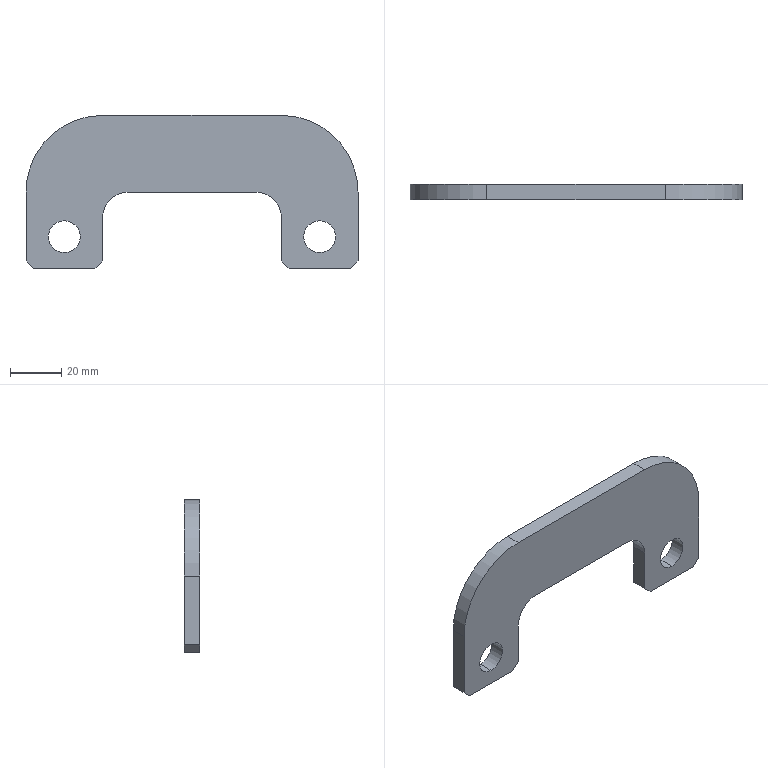Part | SolidWorks | features FlatPattern 1, SMBaseFlange 1, SheetMetal 1 | 1 solid | 22 faces | box 130 x 6 x 60 mm | volume 30559 mm3 | plane 14 | cylinder 8 | commonest cylinder face diameters 12.5 x4 20 x2 60 x2
STEP:
#1=CARTESIAN_POINT('',(15.,-6.,6.25));
#2=VERTEX_POINT('',#1);
#3=CARTESIAN_POINT('',(15.,-6.,18.75));
#4=VERTEX_POINT('',#3);
#5=CARTESIAN_POINT('',(15.,-6.,12.5));
#6=DIRECTION('',(0.,1.,0.));
#7=DIRECTION('',(0.,0.,1.));
#8=AXIS2_PLACEMENT_3D('',#5,#6,#7);
#9=CIRCLE('',#8,6.25);
#10=EDGE_CURVE('',#2,#4,#9,.T.);
#11=ORIENTED_EDGE('',*,*,#10,.F.);
#12=CARTESIAN_POINT('',(15.,0.,6.25));
#13=VERTEX_POINT('',#12);
#14=CARTESIAN_POINT('',(15.,-6.,6.25));
#15=DIRECTION('',(0.,1.,0.));
#16=VECTOR('',#15,1000.);
#17=LINE('',#14,#16);
#18=EDGE_CURVE('',#2,#13,#17,.T.);
#19=ORIENTED_EDGE('',*,*,#18,.T.);
#20=CARTESIAN_POINT('',(15.,0.,18.75));
#21=VERTEX_POINT('',#20);
#22=CARTESIAN_POINT('',(15.,0.,12.5));
#23=DIRECTION('',(0.,1.,0.));
#24=DIRECTION('',(0.,0.,1.));
#25=AXIS2_PLACEMENT_3D('',#22,#23,#24);
#26=CIRCLE('',#25,6.25);
#27=EDGE_CURVE('',#13,#21,#26,.T.);
#28=ORIENTED_EDGE('',*,*,#27,.T.);
#29=CARTESIAN_POINT('',(15.,-6.,18.75));
#30=DIRECTION('',(0.,1.,0.));
#31=VECTOR('',#30,1000.);
#32=LINE('',#29,#31);
#33=EDGE_CURVE('',#4,#21,#32,.T.);
#34=ORIENTED_EDGE('',*,*,#33,.F.);
#35=EDGE_LOOP('',(#11,#19,#28,#34));
#36=FACE_OUTER_BOUND('',#35,.T.);
#37=CARTESIAN_POINT('',(15.,-6.,12.5));
#38=DIRECTION('',(0.,1.,0.));
#39=DIRECTION('',(0.,0.,1.));
#40=AXIS2_PLACEMENT_3D('',#37,#38,#39);
#41=CYLINDRICAL_SURFACE('',#40,6.25);
#42=ADVANCED_FACE('',(#36),#41,.F.);
#43=CARTESIAN_POINT('',(115.,-6.,6.25));
#44=VERTEX_POINT('',#43);
#45=CARTESIAN_POINT('',(115.,-6.,18.75));
#46=VERTEX_POINT('',#45);
#47=CARTESIAN_POINT('',(115.,-6.,12.5));
#48=DIRECTION('',(0.,1.,0.));
#49=DIRECTION('',(0.,0.,1.));
#50=AXIS2_PLACEMENT_3D('',#47,#48,#49);
#51=CIRCLE('',#50,6.25);
#52=EDGE_CURVE('',#44,#46,#51,.T.);
#53=ORIENTED_EDGE('',*,*,#52,.F.);
#54=CARTESIAN_POINT('',(115.,0.,6.25));
#55=VERTEX_POINT('',#54);
#56=CARTESIAN_POINT('',(115.,-6.,6.25));
#57=DIRECTION('',(0.,1.,0.));
#58=VECTOR('',#57,1000.);
#59=LINE('',#56,#58);
#60=EDGE_CURVE('',#44,#55,#59,.T.);
#61=ORIENTED_EDGE('',*,*,#60,.T.);
#62=CARTESIAN_POINT('',(115.,0.,18.75));
#63=VERTEX_POINT('',#62);
#64=CARTESIAN_POINT('',(115.,0.,12.5));
#65=DIRECTION('',(0.,1.,0.));
#66=DIRECTION('',(0.,0.,1.));
#67=AXIS2_PLACEMENT_3D('',#64,#65,#66);
#68=CIRCLE('',#67,6.25);
#69=EDGE_CURVE('',#55,#63,#68,.T.);
#70=ORIENTED_EDGE('',*,*,#69,.T.);
#71=CARTESIAN_POINT('',(115.,-6.,18.75));
#72=DIRECTION('',(0.,1.,0.));
#73=VECTOR('',#72,1000.);
#74=LINE('',#71,#73);
#75=EDGE_CURVE('',#46,#63,#74,.T.);
#76=ORIENTED_EDGE('',*,*,#75,.F.);
#77=EDGE_LOOP('',(#53,#61,#70,#76));
#78=FACE_OUTER_BOUND('',#77,.T.);
#79=CARTESIAN_POINT('',(115.,-6.,12.5));
#80=DIRECTION('',(0.,1.,0.));
#81=DIRECTION('',(0.,0.,1.));
#82=AXIS2_PLACEMENT_3D('',#79,#80,#81);
#83=CYLINDRICAL_SURFACE('',#82,6.25);
#84=ADVANCED_FACE('',(#78),#83,.F.);
#85=CARTESIAN_POINT('',(100.,0.,20.));
#86=VERTEX_POINT('',#85);
#87=CARTESIAN_POINT('',(90.,0.,30.));
#88=VERTEX_POINT('',#87);
#89=CARTESIAN_POINT('',(90.,0.,20.));
#90=DIRECTION('',(0.,-1.,0.));
#91=DIRECTION('',(0.,0.,-1.));
#92=AXIS2_PLACEMENT_3D('',#89,#90,#91);
#93=CIRCLE('',#92,10.);
#94=EDGE_CURVE('',#86,#88,#93,.T.);
#95=ORIENTED_EDGE('',*,*,#94,.F.);
#96=CARTESIAN_POINT('',(100.,-6.,20.));
#97=VERTEX_POINT('',#96);
#98=CARTESIAN_POINT('',(100.,-6.,20.));
#99=DIRECTION('',(0.,1.,0.));
#100=VECTOR('',#99,1000.);
#101=LINE('',#98,#100);
#102=EDGE_CURVE('',#97,#86,#101,.T.);
#103=ORIENTED_EDGE('',*,*,#102,.F.);
#104=CARTESIAN_POINT('',(90.,-6.,30.));
#105=VERTEX_POINT('',#104);
#106=CARTESIAN_POINT('',(90.,-6.,20.));
#107=DIRECTION('',(0.,-1.,0.));
#108=DIRECTION('',(0.,0.,-1.));
#109=AXIS2_PLACEMENT_3D('',#106,#107,#108);
#110=CIRCLE('',#109,10.);
#111=EDGE_CURVE('',#97,#105,#110,.T.);
#112=ORIENTED_EDGE('',*,*,#111,.T.);
#113=CARTESIAN_POINT('',(90.,-6.,30.));
#114=DIRECTION('',(0.,1.,0.));
#115=VECTOR('',#114,1000.);
#116=LINE('',#113,#115);
#117=EDGE_CURVE('',#105,#88,#116,.T.);
#118=ORIENTED_EDGE('',*,*,#117,.T.);
#119=EDGE_LOOP('',(#95,#103,#112,#118));
#120=FACE_OUTER_BOUND('',#119,.T.);
#121=CARTESIAN_POINT('',(90.,-6.,20.));
#122=DIRECTION('',(0.,1.,0.));
#123=DIRECTION('',(0.,0.,1.));
#124=AXIS2_PLACEMENT_3D('',#121,#122,#123);
#125=CYLINDRICAL_SURFACE('',#124,10.);
#126=ADVANCED_FACE('',(#120),#125,.F.);
#127=CARTESIAN_POINT('',(100.,0.,3.));
#128=VERTEX_POINT('',#127);
#129=CARTESIAN_POINT('',(100.,0.,3.));
#130=DIRECTION('',(0.,0.,1.));
#131=VECTOR('',#130,1000.);
#132=LINE('',#129,#131);
#133=EDGE_CURVE('',#128,#86,#132,.T.);
#134=ORIENTED_EDGE('',*,*,#133,.F.);
#135=CARTESIAN_POINT('',(100.,-6.,3.));
#136=VERTEX_POINT('',#135);
#137=CARTESIAN_POINT('',(100.,-6.,3.));
#138=DIRECTION('',(0.,1.,0.));
#139=VECTOR('',#138,1000.);
#140=LINE('',#137,#139);
#141=EDGE_CURVE('',#136,#128,#140,.T.);
#142=ORIENTED_EDGE('',*,*,#141,.F.);
#143=CARTESIAN_POINT('',(100.,-6.,3.));
#144=DIRECTION('',(0.,0.,1.));
#145=VECTOR('',#144,1000.);
#146=LINE('',#143,#145);
#147=EDGE_CURVE('',#136,#97,#146,.T.);
#148=ORIENTED_EDGE('',*,*,#147,.T.);
#149=ORIENTED_EDGE('',*,*,#102,.T.);
#150=EDGE_LOOP('',(#134,#142,#148,#149));
#151=FACE_OUTER_BOUND('',#150,.T.);
#152=CARTESIAN_POINT('',(100.,-6.,3.));
#153=DIRECTION('',(-1.,0.,0.));
#154=DIRECTION('',(0.,0.,1.));
#155=AXIS2_PLACEMENT_3D('',#152,#153,#154);
#156=PLANE('',#155);
#157=ADVANCED_FACE('',(#151),#156,.T.);
#158=CARTESIAN_POINT('',(103.,0.,0.));
#159=VERTEX_POINT('',#158);
#160=CARTESIAN_POINT('',(103.,0.,0.));
#161=DIRECTION('',(-0.7071,0.,0.7071));
#162=VECTOR('',#161,1000.);
#163=LINE('',#160,#162);
#164=EDGE_CURVE('',#159,#128,#163,.T.);
#165=ORIENTED_EDGE('',*,*,#164,.F.);
#166=CARTESIAN_POINT('',(103.,-6.,0.));
#167=VERTEX_POINT('',#166);
#168=CARTESIAN_POINT('',(103.,-6.,0.));
#169=DIRECTION('',(0.,1.,0.));
#170=VECTOR('',#169,1000.);
#171=LINE('',#168,#170);
#172=EDGE_CURVE('',#167,#159,#171,.T.);
#173=ORIENTED_EDGE('',*,*,#172,.F.);
#174=CARTESIAN_POINT('',(103.,-6.,0.));
#175=DIRECTION('',(-0.7071,0.,0.7071));
#176=VECTOR('',#175,1000.);
#177=LINE('',#174,#176);
#178=EDGE_CURVE('',#167,#136,#177,.T.);
#179=ORIENTED_EDGE('',*,*,#178,.T.);
#180=ORIENTED_EDGE('',*,*,#141,.T.);
#181=EDGE_LOOP('',(#165,#173,#179,#180));
#182=FACE_OUTER_BOUND('',#181,.T.);
#183=CARTESIAN_POINT('',(103.,-6.,0.));
#184=DIRECTION('',(-0.7071,0.,-0.7071));
#185=DIRECTION('',(-0.7071,0.,0.7071));
#186=AXIS2_PLACEMENT_3D('',#183,#184,#185);
#187=PLANE('',#186);
#188=ADVANCED_FACE('',(#182),#187,.T.);
#189=CARTESIAN_POINT('',(127.,0.,0.));
#190=VERTEX_POINT('',#189);
#191=CARTESIAN_POINT('',(127.,0.,0.));
#192=DIRECTION('',(-1.,0.,0.));
#193=VECTOR('',#192,1000.);
#194=LINE('',#191,#193);
#195=EDGE_CURVE('',#190,#159,#194,.T.);
#196=ORIENTED_EDGE('',*,*,#195,.F.);
#197=CARTESIAN_POINT('',(127.,-6.,0.));
#198=VERTEX_POINT('',#197);
#199=CARTESIAN_POINT('',(127.,-6.,0.));
#200=DIRECTION('',(0.,1.,0.));
#201=VECTOR('',#200,1000.);
#202=LINE('',#199,#201);
#203=EDGE_CURVE('',#198,#190,#202,.T.);
#204=ORIENTED_EDGE('',*,*,#203,.F.);
#205=CARTESIAN_POINT('',(127.,-6.,0.));
#206=DIRECTION('',(-1.,0.,0.));
#207=VECTOR('',#206,1000.);
#208=LINE('',#205,#207);
#209=EDGE_CURVE('',#198,#167,#208,.T.);
#210=ORIENTED_EDGE('',*,*,#209,.T.);
#211=ORIENTED_EDGE('',*,*,#172,.T.);
#212=EDGE_LOOP('',(#196,#204,#210,#211));
#213=FACE_OUTER_BOUND('',#212,.T.);
#214=CARTESIAN_POINT('',(127.,-6.,0.));
#215=DIRECTION('',(0.,0.,-1.));
#216=DIRECTION('',(-1.,0.,0.));
#217=AXIS2_PLACEMENT_3D('',#214,#215,#216);
#218=PLANE('',#217);
#219=ADVANCED_FACE('',(#213),#218,.T.);
#220=CARTESIAN_POINT('',(130.,0.,3.));
#221=VERTEX_POINT('',#220);
#222=CARTESIAN_POINT('',(130.,0.,3.));
#223=DIRECTION('',(-0.7071,0.,-0.7071));
#224=VECTOR('',#223,1000.);
#225=LINE('',#222,#224);
#226=EDGE_CURVE('',#221,#190,#225,.T.);
#227=ORIENTED_EDGE('',*,*,#226,.F.);
#228=CARTESIAN_POINT('',(130.,-6.,3.));
#229=VERTEX_POINT('',#228);
#230=CARTESIAN_POINT('',(130.,-6.,3.));
#231=DIRECTION('',(0.,1.,0.));
#232=VECTOR('',#231,1000.);
#233=LINE('',#230,#232);
#234=EDGE_CURVE('',#229,#221,#233,.T.);
#235=ORIENTED_EDGE('',*,*,#234,.F.);
#236=CARTESIAN_POINT('',(130.,-6.,3.));
#237=DIRECTION('',(-0.7071,0.,-0.7071));
#238=VECTOR('',#237,1000.);
#239=LINE('',#236,#238);
#240=EDGE_CURVE('',#229,#198,#239,.T.);
#241=ORIENTED_EDGE('',*,*,#240,.T.);
#242=ORIENTED_EDGE('',*,*,#203,.T.);
#243=EDGE_LOOP('',(#227,#235,#241,#242));
#244=FACE_OUTER_BOUND('',#243,.T.);
#245=CARTESIAN_POINT('',(130.,-6.,3.));
#246=DIRECTION('',(0.7071,0.,-0.7071));
#247=DIRECTION('',(-0.7071,0.,-0.7071));
#248=AXIS2_PLACEMENT_3D('',#245,#246,#247);
#249=PLANE('',#248);
#250=ADVANCED_FACE('',(#244),#249,.T.);
#251=CARTESIAN_POINT('',(130.,0.,30.));
#252=VERTEX_POINT('',#251);
#253=CARTESIAN_POINT('',(130.,0.,30.));
#254=DIRECTION('',(0.,0.,-1.));
#255=VECTOR('',#254,1000.);
#256=LINE('',#253,#255);
#257=EDGE_CURVE('',#252,#221,#256,.T.);
#258=ORIENTED_EDGE('',*,*,#257,.F.);
#259=CARTESIAN_POINT('',(130.,-6.,30.));
#260=VERTEX_POINT('',#259);
#261=CARTESIAN_POINT('',(130.,-6.,30.));
#262=DIRECTION('',(0.,1.,0.));
#263=VECTOR('',#262,1000.);
#264=LINE('',#261,#263);
#265=EDGE_CURVE('',#260,#252,#264,.T.);
#266=ORIENTED_EDGE('',*,*,#265,.F.);
#267=CARTESIAN_POINT('',(130.,-6.,30.));
#268=DIRECTION('',(0.,0.,-1.));
#269=VECTOR('',#268,1000.);
#270=LINE('',#267,#269);
#271=EDGE_CURVE('',#260,#229,#270,.T.);
#272=ORIENTED_EDGE('',*,*,#271,.T.);
#273=ORIENTED_EDGE('',*,*,#234,.T.);
#274=EDGE_LOOP('',(#258,#266,#272,#273));
#275=FACE_OUTER_BOUND('',#274,.T.);
#276=CARTESIAN_POINT('',(130.,-6.,30.));
#277=DIRECTION('',(1.,0.,0.));
#278=DIRECTION('',(0.,0.,-1.));
#279=AXIS2_PLACEMENT_3D('',#276,#277,#278);
#280=PLANE('',#279);
#281=ADVANCED_FACE('',(#275),#280,.T.);
#282=CARTESIAN_POINT('',(100.,0.,60.));
#283=VERTEX_POINT('',#282);
#284=CARTESIAN_POINT('',(100.,0.,30.));
#285=DIRECTION('',(0.,1.,0.));
#286=DIRECTION('',(0.,0.,1.));
#287=AXIS2_PLACEMENT_3D('',#284,#285,#286);
#288=CIRCLE('',#287,30.);
#289=EDGE_CURVE('',#283,#252,#288,.T.);
#290=ORIENTED_EDGE('',*,*,#289,.F.);
#291=CARTESIAN_POINT('',(100.,-6.,60.));
#292=VERTEX_POINT('',#291);
#293=CARTESIAN_POINT('',(100.,-6.,60.));
#294=DIRECTION('',(0.,1.,0.));
#295=VECTOR('',#294,1000.);
#296=LINE('',#293,#295);
#297=EDGE_CURVE('',#292,#283,#296,.T.);
#298=ORIENTED_EDGE('',*,*,#297,.F.);
#299=CARTESIAN_POINT('',(100.,-6.,30.));
#300=DIRECTION('',(0.,1.,0.));
#301=DIRECTION('',(0.,0.,1.));
#302=AXIS2_PLACEMENT_3D('',#299,#300,#301);
#303=CIRCLE('',#302,30.);
#304=EDGE_CURVE('',#292,#260,#303,.T.);
#305=ORIENTED_EDGE('',*,*,#304,.T.);
#306=ORIENTED_EDGE('',*,*,#265,.T.);
#307=EDGE_LOOP('',(#290,#298,#305,#306));
#308=FACE_OUTER_BOUND('',#307,.T.);
#309=CARTESIAN_POINT('',(100.,-6.,30.));
#310=DIRECTION('',(0.,1.,0.));
#311=DIRECTION('',(0.,0.,1.));
#312=AXIS2_PLACEMENT_3D('',#309,#310,#311);
#313=CYLINDRICAL_SURFACE('',#312,30.);
#314=ADVANCED_FACE('',(#308),#313,.T.);
#315=CARTESIAN_POINT('',(30.,0.,60.));
#316=VERTEX_POINT('',#315);
#317=CARTESIAN_POINT('',(30.,0.,60.));
#318=DIRECTION('',(1.,0.,0.));
#319=VECTOR('',#318,1000.);
#320=LINE('',#317,#319);
#321=EDGE_CURVE('',#316,#283,#320,.T.);
#322=ORIENTED_EDGE('',*,*,#321,.F.);
#323=CARTESIAN_POINT('',(30.,-6.,60.));
#324=VERTEX_POINT('',#323);
#325=CARTESIAN_POINT('',(30.,-6.,60.));
#326=DIRECTION('',(0.,1.,0.));
#327=VECTOR('',#326,1000.);
#328=LINE('',#325,#327);
#329=EDGE_CURVE('',#324,#316,#328,.T.);
#330=ORIENTED_EDGE('',*,*,#329,.F.);
#331=CARTESIAN_POINT('',(30.,-6.,60.));
#332=DIRECTION('',(1.,0.,0.));
#333=VECTOR('',#332,1000.);
#334=LINE('',#331,#333);
#335=EDGE_CURVE('',#324,#292,#334,.T.);
#336=ORIENTED_EDGE('',*,*,#335,.T.);
#337=ORIENTED_EDGE('',*,*,#297,.T.);
#338=EDGE_LOOP('',(#322,#330,#336,#337));
#339=FACE_OUTER_BOUND('',#338,.T.);
#340=CARTESIAN_POINT('',(30.,-6.,60.));
#341=DIRECTION('',(0.,0.,1.));
#342=DIRECTION('',(1.,0.,0.));
#343=AXIS2_PLACEMENT_3D('',#340,#341,#342);
#344=PLANE('',#343);
#345=ADVANCED_FACE('',(#339),#344,.T.);
#346=CARTESIAN_POINT('',(0.,0.,30.));
#347=VERTEX_POINT('',#346);
#348=CARTESIAN_POINT('',(30.,0.,30.));
#349=DIRECTION('',(0.,1.,0.));
#350=DIRECTION('',(0.,0.,1.));
#351=AXIS2_PLACEMENT_3D('',#348,#349,#350);
#352=CIRCLE('',#351,30.);
#353=EDGE_CURVE('',#347,#316,#352,.T.);
#354=ORIENTED_EDGE('',*,*,#353,.F.);
#355=CARTESIAN_POINT('',(0.,-6.,30.));
#356=VERTEX_POINT('',#355);
#357=CARTESIAN_POINT('',(0.,-6.,30.));
#358=DIRECTION('',(0.,1.,0.));
#359=VECTOR('',#358,1000.);
#360=LINE('',#357,#359);
#361=EDGE_CURVE('',#356,#347,#360,.T.);
#362=ORIENTED_EDGE('',*,*,#361,.F.);
#363=CARTESIAN_POINT('',(30.,-6.,30.));
#364=DIRECTION('',(0.,1.,0.));
#365=DIRECTION('',(0.,0.,1.));
#366=AXIS2_PLACEMENT_3D('',#363,#364,#365);
#367=CIRCLE('',#366,30.);
#368=EDGE_CURVE('',#356,#324,#367,.T.);
#369=ORIENTED_EDGE('',*,*,#368,.T.);
#370=ORIENTED_EDGE('',*,*,#329,.T.);
#371=EDGE_LOOP('',(#354,#362,#369,#370));
#372=FACE_OUTER_BOUND('',#371,.T.);
#373=CARTESIAN_POINT('',(30.,-6.,30.));
#374=DIRECTION('',(0.,1.,0.));
#375=DIRECTION('',(0.,0.,1.));
#376=AXIS2_PLACEMENT_3D('',#373,#374,#375);
#377=CYLINDRICAL_SURFACE('',#376,30.);
#378=ADVANCED_FACE('',(#372),#377,.T.);
#379=CARTESIAN_POINT('',(0.,0.,3.));
#380=VERTEX_POINT('',#379);
#381=CARTESIAN_POINT('',(0.,0.,3.));
#382=DIRECTION('',(0.,0.,1.));
#383=VECTOR('',#382,1000.);
#384=LINE('',#381,#383);
#385=EDGE_CURVE('',#380,#347,#384,.T.);
#386=ORIENTED_EDGE('',*,*,#385,.F.);
#387=CARTESIAN_POINT('',(0.,-6.,3.));
#388=VERTEX_POINT('',#387);
#389=CARTESIAN_POINT('',(0.,-6.,3.));
#390=DIRECTION('',(0.,1.,0.));
#391=VECTOR('',#390,1000.);
#392=LINE('',#389,#391);
#393=EDGE_CURVE('',#388,#380,#392,.T.);
#394=ORIENTED_EDGE('',*,*,#393,.F.);
#395=CARTESIAN_POINT('',(0.,-6.,3.));
#396=DIRECTION('',(0.,0.,1.));
#397=VECTOR('',#396,1000.);
#398=LINE('',#395,#397);
#399=EDGE_CURVE('',#388,#356,#398,.T.);
#400=ORIENTED_EDGE('',*,*,#399,.T.);
#401=ORIENTED_EDGE('',*,*,#361,.T.);
#402=EDGE_LOOP('',(#386,#394,#400,#401));
#403=FACE_OUTER_BOUND('',#402,.T.);
#404=CARTESIAN_POINT('',(0.,-6.,3.));
#405=DIRECTION('',(-1.,0.,0.));
#406=DIRECTION('',(0.,0.,1.));
#407=AXIS2_PLACEMENT_3D('',#404,#405,#406);
#408=PLANE('',#407);
#409=ADVANCED_FACE('',(#403),#408,.T.);
#410=CARTESIAN_POINT('',(3.,0.,0.));
#411=VERTEX_POINT('',#410);
#412=CARTESIAN_POINT('',(3.,0.,0.));
#413=DIRECTION('',(-0.7071,0.,0.7071));
#414=VECTOR('',#413,1000.);
#415=LINE('',#412,#414);
#416=EDGE_CURVE('',#411,#380,#415,.T.);
#417=ORIENTED_EDGE('',*,*,#416,.F.);
#418=CARTESIAN_POINT('',(3.,-6.,0.));
#419=VERTEX_POINT('',#418);
#420=CARTESIAN_POINT('',(3.,-6.,0.));
#421=DIRECTION('',(0.,1.,0.));
#422=VECTOR('',#421,1000.);
#423=LINE('',#420,#422);
#424=EDGE_CURVE('',#419,#411,#423,.T.);
#425=ORIENTED_EDGE('',*,*,#424,.F.);
#426=CARTESIAN_POINT('',(3.,-6.,0.));
#427=DIRECTION('',(-0.7071,0.,0.7071));
#428=VECTOR('',#427,1000.);
#429=LINE('',#426,#428);
#430=EDGE_CURVE('',#419,#388,#429,.T.);
#431=ORIENTED_EDGE('',*,*,#430,.T.);
#432=ORIENTED_EDGE('',*,*,#393,.T.);
#433=EDGE_LOOP('',(#417,#425,#431,#432));
#434=FACE_OUTER_BOUND('',#433,.T.);
#435=CARTESIAN_POINT('',(3.,-6.,0.));
#436=DIRECTION('',(-0.7071,0.,-0.7071));
#437=DIRECTION('',(-0.7071,0.,0.7071));
#438=AXIS2_PLACEMENT_3D('',#435,#436,#437);
#439=PLANE('',#438);
#440=ADVANCED_FACE('',(#434),#439,.T.);
#441=CARTESIAN_POINT('',(27.,0.,0.));
#442=VERTEX_POINT('',#441);
#443=CARTESIAN_POINT('',(27.,0.,0.));
#444=DIRECTION('',(-1.,0.,0.));
#445=VECTOR('',#444,1000.);
#446=LINE('',#443,#445);
#447=EDGE_CURVE('',#442,#411,#446,.T.);
#448=ORIENTED_EDGE('',*,*,#447,.F.);
#449=CARTESIAN_POINT('',(27.,-6.,0.));
#450=VERTEX_POINT('',#449);
#451=CARTESIAN_POINT('',(27.,-6.,0.));
#452=DIRECTION('',(0.,1.,0.));
#453=VECTOR('',#452,1000.);
#454=LINE('',#451,#453);
#455=EDGE_CURVE('',#450,#442,#454,.T.);
#456=ORIENTED_EDGE('',*,*,#455,.F.);
#457=CARTESIAN_POINT('',(27.,-6.,0.));
#458=DIRECTION('',(-1.,0.,0.));
#459=VECTOR('',#458,1000.);
#460=LINE('',#457,#459);
#461=EDGE_CURVE('',#450,#419,#460,.T.);
#462=ORIENTED_EDGE('',*,*,#461,.T.);
#463=ORIENTED_EDGE('',*,*,#424,.T.);
#464=EDGE_LOOP('',(#448,#456,#462,#463));
#465=FACE_OUTER_BOUND('',#464,.T.);
#466=CARTESIAN_POINT('',(27.,-6.,0.));
#467=DIRECTION('',(0.,0.,-1.));
#468=DIRECTION('',(-1.,0.,0.));
#469=AXIS2_PLACEMENT_3D('',#466,#467,#468);
#470=PLANE('',#469);
#471=ADVANCED_FACE('',(#465),#470,.T.);
#472=CARTESIAN_POINT('',(30.,0.,3.));
#473=VERTEX_POINT('',#472);
#474=CARTESIAN_POINT('',(30.,0.,3.));
#475=DIRECTION('',(-0.7071,0.,-0.7071));
#476=VECTOR('',#475,1000.);
#477=LINE('',#474,#476);
#478=EDGE_CURVE('',#473,#442,#477,.T.);
#479=ORIENTED_EDGE('',*,*,#478,.F.);
#480=CARTESIAN_POINT('',(30.,-6.,3.));
#481=VERTEX_POINT('',#480);
#482=CARTESIAN_POINT('',(30.,-6.,3.));
#483=DIRECTION('',(0.,1.,0.));
#484=VECTOR('',#483,1000.);
#485=LINE('',#482,#484);
#486=EDGE_CURVE('',#481,#473,#485,.T.);
#487=ORIENTED_EDGE('',*,*,#486,.F.);
#488=CARTESIAN_POINT('',(30.,-6.,3.));
#489=DIRECTION('',(-0.7071,0.,-0.7071));
#490=VECTOR('',#489,1000.);
#491=LINE('',#488,#490);
#492=EDGE_CURVE('',#481,#450,#491,.T.);
#493=ORIENTED_EDGE('',*,*,#492,.T.);
#494=ORIENTED_EDGE('',*,*,#455,.T.);
#495=EDGE_LOOP('',(#479,#487,#493,#494));
#496=FACE_OUTER_BOUND('',#495,.T.);
#497=CARTESIAN_POINT('',(30.,-6.,3.));
#498=DIRECTION('',(0.7071,0.,-0.7071));
#499=DIRECTION('',(-0.7071,0.,-0.7071));
#500=AXIS2_PLACEMENT_3D('',#497,#498,#499);
#501=PLANE('',#500);
#502=ADVANCED_FACE('',(#496),#501,.T.);
#503=CARTESIAN_POINT('',(30.,0.,20.));
#504=VERTEX_POINT('',#503);
#505=CARTESIAN_POINT('',(30.,0.,20.));
#506=DIRECTION('',(0.,0.,-1.));
#507=VECTOR('',#506,1000.);
#508=LINE('',#505,#507);
#509=EDGE_CURVE('',#504,#473,#508,.T.);
#510=ORIENTED_EDGE('',*,*,#509,.F.);
#511=CARTESIAN_POINT('',(30.,-6.,20.));
#512=VERTEX_POINT('',#511);
#513=CARTESIAN_POINT('',(30.,-6.,20.));
#514=DIRECTION('',(0.,1.,0.));
#515=VECTOR('',#514,1000.);
#516=LINE('',#513,#515);
#517=EDGE_CURVE('',#512,#504,#516,.T.);
#518=ORIENTED_EDGE('',*,*,#517,.F.);
#519=CARTESIAN_POINT('',(30.,-6.,20.));
#520=DIRECTION('',(0.,0.,-1.));
#521=VECTOR('',#520,1000.);
#522=LINE('',#519,#521);
#523=EDGE_CURVE('',#512,#481,#522,.T.);
#524=ORIENTED_EDGE('',*,*,#523,.T.);
#525=ORIENTED_EDGE('',*,*,#486,.T.);
#526=EDGE_LOOP('',(#510,#518,#524,#525));
#527=FACE_OUTER_BOUND('',#526,.T.);
#528=CARTESIAN_POINT('',(30.,-6.,20.));
#529=DIRECTION('',(1.,0.,0.));
#530=DIRECTION('',(0.,0.,-1.));
#531=AXIS2_PLACEMENT_3D('',#528,#529,#530);
#532=PLANE('',#531);
#533=ADVANCED_FACE('',(#527),#532,.T.);
#534=CARTESIAN_POINT('',(40.,0.,30.));
#535=VERTEX_POINT('',#534);
#536=CARTESIAN_POINT('',(40.,0.,20.));
#537=DIRECTION('',(0.,-1.,0.));
#538=DIRECTION('',(0.,0.,-1.));
#539=AXIS2_PLACEMENT_3D('',#536,#537,#538);
#540=CIRCLE('',#539,10.);
#541=EDGE_CURVE('',#535,#504,#540,.T.);
#542=ORIENTED_EDGE('',*,*,#541,.F.);
#543=CARTESIAN_POINT('',(40.,-6.,30.));
#544=VERTEX_POINT('',#543);
#545=CARTESIAN_POINT('',(40.,-6.,30.));
#546=DIRECTION('',(0.,1.,0.));
#547=VECTOR('',#546,1000.);
#548=LINE('',#545,#547);
#549=EDGE_CURVE('',#544,#535,#548,.T.);
#550=ORIENTED_EDGE('',*,*,#549,.F.);
#551=CARTESIAN_POINT('',(40.,-6.,20.));
#552=DIRECTION('',(0.,-1.,0.));
#553=DIRECTION('',(0.,0.,-1.));
#554=AXIS2_PLACEMENT_3D('',#551,#552,#553);
#555=CIRCLE('',#554,10.);
#556=EDGE_CURVE('',#544,#512,#555,.T.);
#557=ORIENTED_EDGE('',*,*,#556,.T.);
#558=ORIENTED_EDGE('',*,*,#517,.T.);
#559=EDGE_LOOP('',(#542,#550,#557,#558));
#560=FACE_OUTER_BOUND('',#559,.T.);
#561=CARTESIAN_POINT('',(40.,-6.,20.));
#562=DIRECTION('',(0.,1.,0.));
#563=DIRECTION('',(0.,0.,1.));
#564=AXIS2_PLACEMENT_3D('',#561,#562,#563);
#565=CYLINDRICAL_SURFACE('',#564,10.);
#566=ADVANCED_FACE('',(#560),#565,.F.);
#567=CARTESIAN_POINT('',(90.,0.,30.));
#568=DIRECTION('',(-1.,0.,0.));
#569=VECTOR('',#568,1000.);
#570=LINE('',#567,#569);
#571=EDGE_CURVE('',#88,#535,#570,.T.);
#572=ORIENTED_EDGE('',*,*,#571,.F.);
#573=ORIENTED_EDGE('',*,*,#117,.F.);
#574=CARTESIAN_POINT('',(90.,-6.,30.));
#575=DIRECTION('',(-1.,0.,0.));
#576=VECTOR('',#575,1000.);
#577=LINE('',#574,#576);
#578=EDGE_CURVE('',#105,#544,#577,.T.);
#579=ORIENTED_EDGE('',*,*,#578,.T.);
#580=ORIENTED_EDGE('',*,*,#549,.T.);
#581=EDGE_LOOP('',(#572,#573,#579,#580));
#582=FACE_OUTER_BOUND('',#581,.T.);
#583=CARTESIAN_POINT('',(90.,-6.,30.));
#584=DIRECTION('',(0.,0.,-1.));
#585=DIRECTION('',(-1.,0.,0.));
#586=AXIS2_PLACEMENT_3D('',#583,#584,#585);
#587=PLANE('',#586);
#588=ADVANCED_FACE('',(#582),#587,.T.);
#589=CARTESIAN_POINT('',(15.,-6.,12.5));
#590=DIRECTION('',(0.,1.,0.));
#591=DIRECTION('',(0.,0.,1.));
#592=AXIS2_PLACEMENT_3D('',#589,#590,#591);
#593=CIRCLE('',#592,6.25);
#594=EDGE_CURVE('',#4,#2,#593,.T.);
#595=ORIENTED_EDGE('',*,*,#594,.T.);
#596=ORIENTED_EDGE('',*,*,#10,.T.);
#597=EDGE_LOOP('',(#595,#596));
#598=FACE_BOUND('',#597,.T.);
#599=CARTESIAN_POINT('',(115.,-6.,12.5));
#600=DIRECTION('',(0.,1.,0.));
#601=DIRECTION('',(0.,0.,1.));
#602=AXIS2_PLACEMENT_3D('',#599,#600,#601);
#603=CIRCLE('',#602,6.25);
#604=EDGE_CURVE('',#46,#44,#603,.T.);
#605=ORIENTED_EDGE('',*,*,#604,.T.);
#606=ORIENTED_EDGE('',*,*,#52,.T.);
#607=EDGE_LOOP('',(#605,#606));
#608=FACE_BOUND('',#607,.T.);
#609=ORIENTED_EDGE('',*,*,#111,.F.);
#610=ORIENTED_EDGE('',*,*,#147,.F.);
#611=ORIENTED_EDGE('',*,*,#178,.F.);
#612=ORIENTED_EDGE('',*,*,#209,.F.);
#613=ORIENTED_EDGE('',*,*,#240,.F.);
#614=ORIENTED_EDGE('',*,*,#271,.F.);
#615=ORIENTED_EDGE('',*,*,#304,.F.);
#616=ORIENTED_EDGE('',*,*,#335,.F.);
#617=ORIENTED_EDGE('',*,*,#368,.F.);
#618=ORIENTED_EDGE('',*,*,#399,.F.);
#619=ORIENTED_EDGE('',*,*,#430,.F.);
#620=ORIENTED_EDGE('',*,*,#461,.F.);
#621=ORIENTED_EDGE('',*,*,#492,.F.);
#622=ORIENTED_EDGE('',*,*,#523,.F.);
#623=ORIENTED_EDGE('',*,*,#556,.F.);
#624=ORIENTED_EDGE('',*,*,#578,.F.);
#625=EDGE_LOOP('',(#609,#610,#611,#612,#613,#614,#615,#616,#617,#618,#619,#620,#621,#622,#623,#624));
#626=FACE_OUTER_BOUND('',#625,.T.);
#627=CARTESIAN_POINT('',(90.,-6.,20.));
#628=DIRECTION('',(0.,-1.,0.));
#629=DIRECTION('',(0.,0.,-1.));
#630=AXIS2_PLACEMENT_3D('',#627,#628,#629);
#631=PLANE('',#630);
#632=ADVANCED_FACE('',(#598,#608,#626),#631,.T.);
#633=CARTESIAN_POINT('',(15.,0.,12.5));
#634=DIRECTION('',(0.,1.,0.));
#635=DIRECTION('',(0.,0.,1.));
#636=AXIS2_PLACEMENT_3D('',#633,#634,#635);
#637=CIRCLE('',#636,6.25);
#638=EDGE_CURVE('',#21,#13,#637,.T.);
#639=ORIENTED_EDGE('',*,*,#638,.F.);
#640=ORIENTED_EDGE('',*,*,#27,.F.);
#641=EDGE_LOOP('',(#639,#640));
#642=FACE_BOUND('',#641,.T.);
#643=CARTESIAN_POINT('',(115.,0.,12.5));
#644=DIRECTION('',(0.,1.,0.));
#645=DIRECTION('',(0.,0.,1.));
#646=AXIS2_PLACEMENT_3D('',#643,#644,#645);
#647=CIRCLE('',#646,6.25);
#648=EDGE_CURVE('',#63,#55,#647,.T.);
#649=ORIENTED_EDGE('',*,*,#648,.F.);
#650=ORIENTED_EDGE('',*,*,#69,.F.);
#651=EDGE_LOOP('',(#649,#650));
#652=FACE_BOUND('',#651,.T.);
#653=ORIENTED_EDGE('',*,*,#94,.T.);
#654=ORIENTED_EDGE('',*,*,#571,.T.);
#655=ORIENTED_EDGE('',*,*,#541,.T.);
#656=ORIENTED_EDGE('',*,*,#509,.T.);
#657=ORIENTED_EDGE('',*,*,#478,.T.);
#658=ORIENTED_EDGE('',*,*,#447,.T.);
#659=ORIENTED_EDGE('',*,*,#416,.T.);
#660=ORIENTED_EDGE('',*,*,#385,.T.);
#661=ORIENTED_EDGE('',*,*,#353,.T.);
#662=ORIENTED_EDGE('',*,*,#321,.T.);
#663=ORIENTED_EDGE('',*,*,#289,.T.);
#664=ORIENTED_EDGE('',*,*,#257,.T.);
#665=ORIENTED_EDGE('',*,*,#226,.T.);
#666=ORIENTED_EDGE('',*,*,#195,.T.);
#667=ORIENTED_EDGE('',*,*,#164,.T.);
#668=ORIENTED_EDGE('',*,*,#133,.T.);
#669=EDGE_LOOP('',(#653,#654,#655,#656,#657,#658,#659,#660,#661,#662,#663,#664,#665,#666,#667,#668));
#670=FACE_OUTER_BOUND('',#669,.T.);
#671=CARTESIAN_POINT('',(90.,0.,20.));
#672=DIRECTION('',(0.,-1.,0.));
#673=DIRECTION('',(0.,0.,-1.));
#674=AXIS2_PLACEMENT_3D('',#671,#672,#673);
#675=PLANE('',#674);
#676=ADVANCED_FACE('',(#642,#652,#670),#675,.F.);
#677=ORIENTED_EDGE('',*,*,#60,.F.);
#678=ORIENTED_EDGE('',*,*,#604,.F.);
#679=ORIENTED_EDGE('',*,*,#75,.T.);
#680=ORIENTED_EDGE('',*,*,#648,.T.);
#681=EDGE_LOOP('',(#677,#678,#679,#680));
#682=FACE_OUTER_BOUND('',#681,.T.);
#683=CARTESIAN_POINT('',(115.,-6.,12.5));
#684=DIRECTION('',(0.,1.,0.));
#685=DIRECTION('',(0.,0.,1.));
#686=AXIS2_PLACEMENT_3D('',#683,#684,#685);
#687=CYLINDRICAL_SURFACE('',#686,6.25);
#688=ADVANCED_FACE('',(#682),#687,.F.);
#689=ORIENTED_EDGE('',*,*,#18,.F.);
#690=ORIENTED_EDGE('',*,*,#594,.F.);
#691=ORIENTED_EDGE('',*,*,#33,.T.);
#692=ORIENTED_EDGE('',*,*,#638,.T.);
#693=EDGE_LOOP('',(#689,#690,#691,#692));
#694=FACE_OUTER_BOUND('',#693,.T.);
#695=CARTESIAN_POINT('',(15.,-6.,12.5));
#696=DIRECTION('',(0.,1.,0.));
#697=DIRECTION('',(0.,0.,1.));
#698=AXIS2_PLACEMENT_3D('',#695,#696,#697);
#699=CYLINDRICAL_SURFACE('',#698,6.25);
#700=ADVANCED_FACE('',(#694),#699,.F.);
#701=CLOSED_SHELL('',(#42,#84,#126,#157,#188,#219,#250,#281,#314,#345,#378,#409,#440,#471,#502,#533,#566,#588,#632,#676,#688,#700));
#702=MANIFOLD_SOLID_BREP('',#701);
#703=CARTESIAN_POINT('',(0.,0.,0.));
#704=DIRECTION('',(0.,0.,1.));
#705=DIRECTION('',(1.,0.,0.));
#706=AXIS2_PLACEMENT_3D('',#703,#704,#705);
#707=(LENGTH_UNIT()NAMED_UNIT(*)SI_UNIT(.MILLI.,.METRE.));
#708=UNCERTAINTY_MEASURE_WITH_UNIT(LENGTH_MEASURE(0.00001),#707,'','');
#709=(NAMED_UNIT(*)PLANE_ANGLE_UNIT()SI_UNIT($,.RADIAN.));
#710=(NAMED_UNIT(*)SI_UNIT($,.STERADIAN.)SOLID_ANGLE_UNIT());
#711=(GEOMETRIC_REPRESENTATION_CONTEXT(3)GLOBAL_UNCERTAINTY_ASSIGNED_CONTEXT((#708))GLOBAL_UNIT_ASSIGNED_CONTEXT((#707,#709,#710))REPRESENTATION_CONTEXT('',''));
#712=ADVANCED_BREP_SHAPE_REPRESENTATION('',(#702,#706),#711);